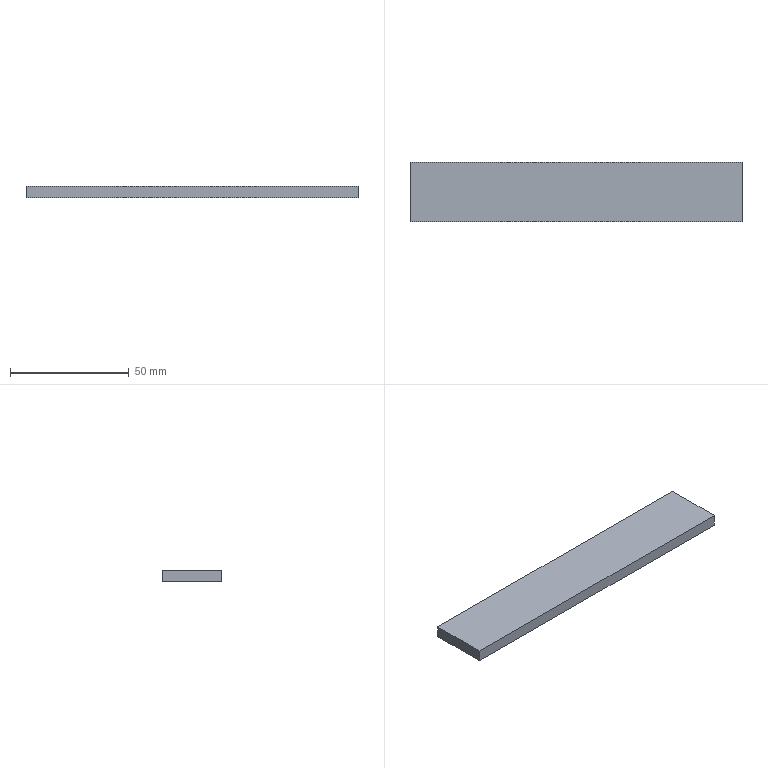Part | SolidWorks | features Extrusion 1 | 1 solid | 6 faces | box 140 x 25 x 5 mm | volume 17500 mm3 | plane 6
STEP:
#1=CARTESIAN_POINT('',(70.,-12.5,0.));
#2=VERTEX_POINT('',#1);
#3=CARTESIAN_POINT('',(70.,12.5,0.));
#4=VERTEX_POINT('',#3);
#5=CARTESIAN_POINT('',(70.,-12.5,0.));
#6=DIRECTION('',(0.,1.,0.));
#7=VECTOR('',#6,1000.);
#8=LINE('',#5,#7);
#9=EDGE_CURVE('',#2,#4,#8,.T.);
#10=ORIENTED_EDGE('',*,*,#9,.T.);
#11=CARTESIAN_POINT('',(70.,12.5,5.));
#12=VERTEX_POINT('',#11);
#13=CARTESIAN_POINT('',(70.,12.5,5.));
#14=DIRECTION('',(0.,0.,-1.));
#15=VECTOR('',#14,1000.);
#16=LINE('',#13,#15);
#17=EDGE_CURVE('',#12,#4,#16,.T.);
#18=ORIENTED_EDGE('',*,*,#17,.F.);
#19=CARTESIAN_POINT('',(70.,-12.5,5.));
#20=VERTEX_POINT('',#19);
#21=CARTESIAN_POINT('',(70.,-12.5,5.));
#22=DIRECTION('',(0.,1.,0.));
#23=VECTOR('',#22,1000.);
#24=LINE('',#21,#23);
#25=EDGE_CURVE('',#20,#12,#24,.T.);
#26=ORIENTED_EDGE('',*,*,#25,.F.);
#27=CARTESIAN_POINT('',(70.,-12.5,5.));
#28=DIRECTION('',(0.,0.,-1.));
#29=VECTOR('',#28,1000.);
#30=LINE('',#27,#29);
#31=EDGE_CURVE('',#20,#2,#30,.T.);
#32=ORIENTED_EDGE('',*,*,#31,.T.);
#33=EDGE_LOOP('',(#10,#18,#26,#32));
#34=FACE_OUTER_BOUND('',#33,.T.);
#35=CARTESIAN_POINT('',(70.,-12.5,5.));
#36=DIRECTION('',(-1.,0.,0.));
#37=DIRECTION('',(0.,0.,1.));
#38=AXIS2_PLACEMENT_3D('',#35,#36,#37);
#39=PLANE('',#38);
#40=ADVANCED_FACE('',(#34),#39,.F.);
#41=CARTESIAN_POINT('',(-70.,12.5,0.));
#42=VERTEX_POINT('',#41);
#43=CARTESIAN_POINT('',(-70.,12.5,0.));
#44=DIRECTION('',(-1.,0.,0.));
#45=VECTOR('',#44,1000.);
#46=LINE('',#43,#45);
#47=EDGE_CURVE('',#4,#42,#46,.T.);
#48=ORIENTED_EDGE('',*,*,#47,.T.);
#49=CARTESIAN_POINT('',(-70.,12.5,5.));
#50=VERTEX_POINT('',#49);
#51=CARTESIAN_POINT('',(-70.,12.5,5.));
#52=DIRECTION('',(0.,0.,-1.));
#53=VECTOR('',#52,1000.);
#54=LINE('',#51,#53);
#55=EDGE_CURVE('',#50,#42,#54,.T.);
#56=ORIENTED_EDGE('',*,*,#55,.F.);
#57=CARTESIAN_POINT('',(-70.,12.5,5.));
#58=DIRECTION('',(-1.,0.,0.));
#59=VECTOR('',#58,1000.);
#60=LINE('',#57,#59);
#61=EDGE_CURVE('',#12,#50,#60,.T.);
#62=ORIENTED_EDGE('',*,*,#61,.F.);
#63=ORIENTED_EDGE('',*,*,#17,.T.);
#64=EDGE_LOOP('',(#48,#56,#62,#63));
#65=FACE_OUTER_BOUND('',#64,.T.);
#66=CARTESIAN_POINT('',(-70.,12.5,5.));
#67=DIRECTION('',(0.,-1.,0.));
#68=DIRECTION('',(0.,0.,-1.));
#69=AXIS2_PLACEMENT_3D('',#66,#67,#68);
#70=PLANE('',#69);
#71=ADVANCED_FACE('',(#65),#70,.F.);
#72=CARTESIAN_POINT('',(-70.,-12.5,0.));
#73=VERTEX_POINT('',#72);
#74=CARTESIAN_POINT('',(-70.,-12.5,0.));
#75=DIRECTION('',(0.,-1.,0.));
#76=VECTOR('',#75,1000.);
#77=LINE('',#74,#76);
#78=EDGE_CURVE('',#42,#73,#77,.T.);
#79=ORIENTED_EDGE('',*,*,#78,.T.);
#80=CARTESIAN_POINT('',(-70.,-12.5,5.));
#81=VERTEX_POINT('',#80);
#82=CARTESIAN_POINT('',(-70.,-12.5,5.));
#83=DIRECTION('',(0.,0.,-1.));
#84=VECTOR('',#83,1000.);
#85=LINE('',#82,#84);
#86=EDGE_CURVE('',#81,#73,#85,.T.);
#87=ORIENTED_EDGE('',*,*,#86,.F.);
#88=CARTESIAN_POINT('',(-70.,-12.5,5.));
#89=DIRECTION('',(0.,-1.,0.));
#90=VECTOR('',#89,1000.);
#91=LINE('',#88,#90);
#92=EDGE_CURVE('',#50,#81,#91,.T.);
#93=ORIENTED_EDGE('',*,*,#92,.F.);
#94=ORIENTED_EDGE('',*,*,#55,.T.);
#95=EDGE_LOOP('',(#79,#87,#93,#94));
#96=FACE_OUTER_BOUND('',#95,.T.);
#97=CARTESIAN_POINT('',(-70.,-12.5,5.));
#98=DIRECTION('',(1.,0.,0.));
#99=DIRECTION('',(0.,0.,-1.));
#100=AXIS2_PLACEMENT_3D('',#97,#98,#99);
#101=PLANE('',#100);
#102=ADVANCED_FACE('',(#96),#101,.F.);
#103=CARTESIAN_POINT('',(-70.,-12.5,0.));
#104=DIRECTION('',(1.,0.,0.));
#105=VECTOR('',#104,1000.);
#106=LINE('',#103,#105);
#107=EDGE_CURVE('',#73,#2,#106,.T.);
#108=ORIENTED_EDGE('',*,*,#107,.T.);
#109=ORIENTED_EDGE('',*,*,#31,.F.);
#110=CARTESIAN_POINT('',(-70.,-12.5,5.));
#111=DIRECTION('',(1.,0.,0.));
#112=VECTOR('',#111,1000.);
#113=LINE('',#110,#112);
#114=EDGE_CURVE('',#81,#20,#113,.T.);
#115=ORIENTED_EDGE('',*,*,#114,.F.);
#116=ORIENTED_EDGE('',*,*,#86,.T.);
#117=EDGE_LOOP('',(#108,#109,#115,#116));
#118=FACE_OUTER_BOUND('',#117,.T.);
#119=CARTESIAN_POINT('',(-70.,-12.5,5.));
#120=DIRECTION('',(0.,1.,0.));
#121=DIRECTION('',(0.,0.,1.));
#122=AXIS2_PLACEMENT_3D('',#119,#120,#121);
#123=PLANE('',#122);
#124=ADVANCED_FACE('',(#118),#123,.F.);
#125=ORIENTED_EDGE('',*,*,#25,.T.);
#126=ORIENTED_EDGE('',*,*,#61,.T.);
#127=ORIENTED_EDGE('',*,*,#92,.T.);
#128=ORIENTED_EDGE('',*,*,#114,.T.);
#129=EDGE_LOOP('',(#125,#126,#127,#128));
#130=FACE_OUTER_BOUND('',#129,.T.);
#131=CARTESIAN_POINT('',(0.,0.,5.));
#132=DIRECTION('',(0.,0.,-1.));
#133=DIRECTION('',(-1.,0.,0.));
#134=AXIS2_PLACEMENT_3D('',#131,#132,#133);
#135=PLANE('',#134);
#136=ADVANCED_FACE('',(#130),#135,.F.);
#137=ORIENTED_EDGE('',*,*,#9,.F.);
#138=ORIENTED_EDGE('',*,*,#107,.F.);
#139=ORIENTED_EDGE('',*,*,#78,.F.);
#140=ORIENTED_EDGE('',*,*,#47,.F.);
#141=EDGE_LOOP('',(#137,#138,#139,#140));
#142=FACE_OUTER_BOUND('',#141,.T.);
#143=CARTESIAN_POINT('',(0.,0.,0.));
#144=DIRECTION('',(0.,0.,-1.));
#145=DIRECTION('',(-1.,0.,0.));
#146=AXIS2_PLACEMENT_3D('',#143,#144,#145);
#147=PLANE('',#146);
#148=ADVANCED_FACE('',(#142),#147,.T.);
#149=CLOSED_SHELL('',(#40,#71,#102,#124,#136,#148));
#150=MANIFOLD_SOLID_BREP('',#149);
#151=CARTESIAN_POINT('',(0.,0.,0.));
#152=DIRECTION('',(0.,0.,1.));
#153=DIRECTION('',(1.,0.,0.));
#154=AXIS2_PLACEMENT_3D('',#151,#152,#153);
#155=(LENGTH_UNIT()NAMED_UNIT(*)SI_UNIT(.MILLI.,.METRE.));
#156=UNCERTAINTY_MEASURE_WITH_UNIT(LENGTH_MEASURE(0.00001),#155,'','');
#157=(NAMED_UNIT(*)PLANE_ANGLE_UNIT()SI_UNIT($,.RADIAN.));
#158=(NAMED_UNIT(*)SI_UNIT($,.STERADIAN.)SOLID_ANGLE_UNIT());
#159=(GEOMETRIC_REPRESENTATION_CONTEXT(3)GLOBAL_UNCERTAINTY_ASSIGNED_CONTEXT((#156))GLOBAL_UNIT_ASSIGNED_CONTEXT((#155,#157,#158))REPRESENTATION_CONTEXT('',''));
#160=ADVANCED_BREP_SHAPE_REPRESENTATION('',(#150,#154),#159);